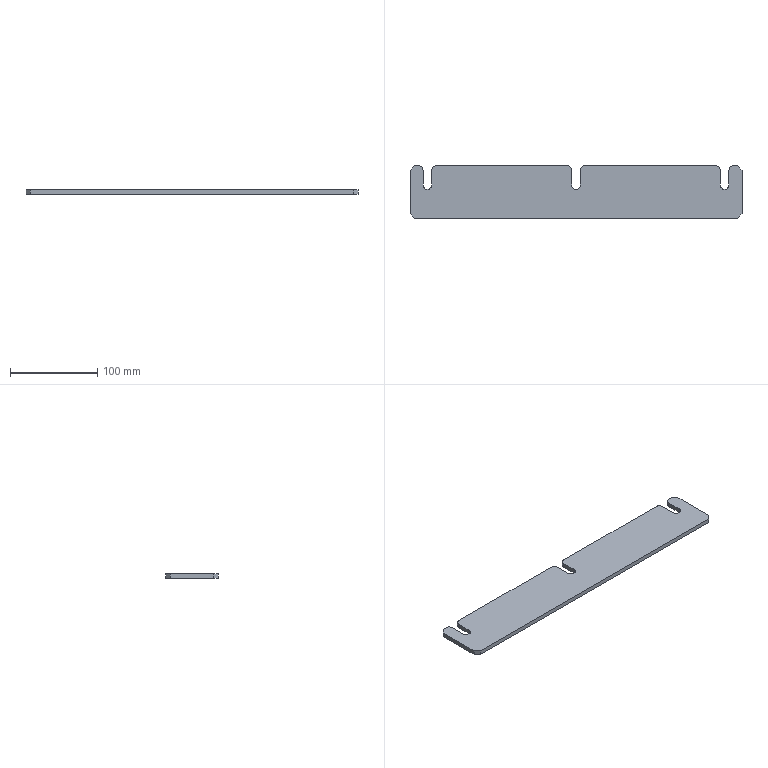Part | SolidWorks | features BaseBody 1 | 1 solid | 28 faces | box 380 x 60 x 5 mm | volume 109700 mm3 | plane 19 | cylinder 9 | commonest cylinder face diameters 10 x9
STEP:
#1=CARTESIAN_POINT('',(-185.,-30.,-5.));
#2=VERTEX_POINT('',#1);
#3=CARTESIAN_POINT('',(-190.,-25.,-5.));
#4=VERTEX_POINT('',#3);
#5=CARTESIAN_POINT('',(-190.,-25.,-5.));
#6=DIRECTION('',(-0.7071,0.7071,0.));
#7=VECTOR('',#6,1000.);
#8=LINE('',#5,#7);
#9=EDGE_CURVE('',#2,#4,#8,.T.);
#10=ORIENTED_EDGE('',*,*,#9,.F.);
#11=CARTESIAN_POINT('',(-185.,-30.,0.));
#12=VERTEX_POINT('',#11);
#13=CARTESIAN_POINT('',(-185.,-30.,-5.));
#14=DIRECTION('',(0.,0.,-1.));
#15=VECTOR('',#14,1000.);
#16=LINE('',#13,#15);
#17=EDGE_CURVE('',#12,#2,#16,.T.);
#18=ORIENTED_EDGE('',*,*,#17,.F.);
#19=CARTESIAN_POINT('',(-190.,-25.,0.));
#20=VERTEX_POINT('',#19);
#21=CARTESIAN_POINT('',(-107.5,-107.5,0.));
#22=DIRECTION('',(0.7071,-0.7071,0.));
#23=VECTOR('',#22,1000.);
#24=LINE('',#21,#23);
#25=EDGE_CURVE('',#20,#12,#24,.T.);
#26=ORIENTED_EDGE('',*,*,#25,.F.);
#27=CARTESIAN_POINT('',(-190.,-25.,-5.));
#28=DIRECTION('',(0.,0.,1.));
#29=VECTOR('',#28,1000.);
#30=LINE('',#27,#29);
#31=EDGE_CURVE('',#4,#20,#30,.T.);
#32=ORIENTED_EDGE('',*,*,#31,.F.);
#33=EDGE_LOOP('',(#10,#18,#26,#32));
#34=FACE_OUTER_BOUND('',#33,.T.);
#35=CARTESIAN_POINT('',(-190.,-25.,-5.));
#36=DIRECTION('',(0.7071,0.7071,0.));
#37=DIRECTION('',(0.,0.,-1.));
#38=AXIS2_PLACEMENT_3D('',#35,#36,#37);
#39=PLANE('',#38);
#40=ADVANCED_FACE('',(#34),#39,.F.);
#41=CARTESIAN_POINT('',(-190.,25.,-5.));
#42=VERTEX_POINT('',#41);
#43=CARTESIAN_POINT('',(-185.,30.,-5.));
#44=VERTEX_POINT('',#43);
#45=CARTESIAN_POINT('',(-185.,30.,-5.));
#46=DIRECTION('',(0.7071,0.7071,0.));
#47=VECTOR('',#46,1000.);
#48=LINE('',#45,#47);
#49=EDGE_CURVE('',#42,#44,#48,.T.);
#50=ORIENTED_EDGE('',*,*,#49,.F.);
#51=CARTESIAN_POINT('',(-190.,25.,0.));
#52=VERTEX_POINT('',#51);
#53=CARTESIAN_POINT('',(-190.,25.,-5.));
#54=DIRECTION('',(0.,0.,-1.));
#55=VECTOR('',#54,1000.);
#56=LINE('',#53,#55);
#57=EDGE_CURVE('',#52,#42,#56,.T.);
#58=ORIENTED_EDGE('',*,*,#57,.F.);
#59=CARTESIAN_POINT('',(-185.,30.,0.));
#60=VERTEX_POINT('',#59);
#61=CARTESIAN_POINT('',(-107.5,107.5,0.));
#62=DIRECTION('',(-0.7071,-0.7071,0.));
#63=VECTOR('',#62,1000.);
#64=LINE('',#61,#63);
#65=EDGE_CURVE('',#60,#52,#64,.T.);
#66=ORIENTED_EDGE('',*,*,#65,.F.);
#67=CARTESIAN_POINT('',(-185.,30.,-5.));
#68=DIRECTION('',(0.,0.,1.));
#69=VECTOR('',#68,1000.);
#70=LINE('',#67,#69);
#71=EDGE_CURVE('',#44,#60,#70,.T.);
#72=ORIENTED_EDGE('',*,*,#71,.F.);
#73=EDGE_LOOP('',(#50,#58,#66,#72));
#74=FACE_OUTER_BOUND('',#73,.T.);
#75=CARTESIAN_POINT('',(-185.,30.,-5.));
#76=DIRECTION('',(0.7071,-0.7071,0.));
#77=DIRECTION('',(0.,0.,-1.));
#78=AXIS2_PLACEMENT_3D('',#75,#76,#77);
#79=PLANE('',#78);
#80=ADVANCED_FACE('',(#74),#79,.F.);
#81=CARTESIAN_POINT('',(190.,-25.,-5.));
#82=VERTEX_POINT('',#81);
#83=CARTESIAN_POINT('',(185.,-30.,-5.));
#84=VERTEX_POINT('',#83);
#85=CARTESIAN_POINT('',(185.,-30.,-5.));
#86=DIRECTION('',(-0.7071,-0.7071,0.));
#87=VECTOR('',#86,1000.);
#88=LINE('',#85,#87);
#89=EDGE_CURVE('',#82,#84,#88,.T.);
#90=ORIENTED_EDGE('',*,*,#89,.F.);
#91=CARTESIAN_POINT('',(190.,-25.,0.));
#92=VERTEX_POINT('',#91);
#93=CARTESIAN_POINT('',(190.,-25.,-5.));
#94=DIRECTION('',(0.,0.,-1.));
#95=VECTOR('',#94,1000.);
#96=LINE('',#93,#95);
#97=EDGE_CURVE('',#92,#82,#96,.T.);
#98=ORIENTED_EDGE('',*,*,#97,.F.);
#99=CARTESIAN_POINT('',(185.,-30.,0.));
#100=VERTEX_POINT('',#99);
#101=CARTESIAN_POINT('',(107.5,-107.5,0.));
#102=DIRECTION('',(0.7071,0.7071,0.));
#103=VECTOR('',#102,1000.);
#104=LINE('',#101,#103);
#105=EDGE_CURVE('',#100,#92,#104,.T.);
#106=ORIENTED_EDGE('',*,*,#105,.F.);
#107=CARTESIAN_POINT('',(185.,-30.,-5.));
#108=DIRECTION('',(0.,0.,1.));
#109=VECTOR('',#108,1000.);
#110=LINE('',#107,#109);
#111=EDGE_CURVE('',#84,#100,#110,.T.);
#112=ORIENTED_EDGE('',*,*,#111,.F.);
#113=EDGE_LOOP('',(#90,#98,#106,#112));
#114=FACE_OUTER_BOUND('',#113,.T.);
#115=CARTESIAN_POINT('',(185.,-30.,-5.));
#116=DIRECTION('',(-0.7071,0.7071,0.));
#117=DIRECTION('',(0.,0.,1.));
#118=AXIS2_PLACEMENT_3D('',#115,#116,#117);
#119=PLANE('',#118);
#120=ADVANCED_FACE('',(#114),#119,.F.);
#121=CARTESIAN_POINT('',(185.,30.,-5.));
#122=VERTEX_POINT('',#121);
#123=CARTESIAN_POINT('',(190.,25.,-5.));
#124=VERTEX_POINT('',#123);
#125=CARTESIAN_POINT('',(190.,25.,-5.));
#126=DIRECTION('',(0.7071,-0.7071,0.));
#127=VECTOR('',#126,1000.);
#128=LINE('',#125,#127);
#129=EDGE_CURVE('',#122,#124,#128,.T.);
#130=ORIENTED_EDGE('',*,*,#129,.F.);
#131=CARTESIAN_POINT('',(185.,30.,0.));
#132=VERTEX_POINT('',#131);
#133=CARTESIAN_POINT('',(185.,30.,-5.));
#134=DIRECTION('',(0.,0.,-1.));
#135=VECTOR('',#134,1000.);
#136=LINE('',#133,#135);
#137=EDGE_CURVE('',#132,#122,#136,.T.);
#138=ORIENTED_EDGE('',*,*,#137,.F.);
#139=CARTESIAN_POINT('',(190.,25.,0.));
#140=VERTEX_POINT('',#139);
#141=CARTESIAN_POINT('',(107.5,107.5,0.));
#142=DIRECTION('',(-0.7071,0.7071,0.));
#143=VECTOR('',#142,1000.);
#144=LINE('',#141,#143);
#145=EDGE_CURVE('',#140,#132,#144,.T.);
#146=ORIENTED_EDGE('',*,*,#145,.F.);
#147=CARTESIAN_POINT('',(190.,25.,-5.));
#148=DIRECTION('',(0.,0.,1.));
#149=VECTOR('',#148,1000.);
#150=LINE('',#147,#149);
#151=EDGE_CURVE('',#124,#140,#150,.T.);
#152=ORIENTED_EDGE('',*,*,#151,.F.);
#153=EDGE_LOOP('',(#130,#138,#146,#152));
#154=FACE_OUTER_BOUND('',#153,.T.);
#155=CARTESIAN_POINT('',(190.,25.,-5.));
#156=DIRECTION('',(-0.7071,-0.7071,0.));
#157=DIRECTION('',(-0.7071,0.7071,0.));
#158=AXIS2_PLACEMENT_3D('',#155,#156,#157);
#159=PLANE('',#158);
#160=ADVANCED_FACE('',(#154),#159,.F.);
#161=CARTESIAN_POINT('',(-165.,25.,-5.));
#162=VERTEX_POINT('',#161);
#163=CARTESIAN_POINT('',(-160.,30.,-5.));
#164=VERTEX_POINT('',#163);
#165=CARTESIAN_POINT('',(-160.,25.,-5.));
#166=DIRECTION('',(0.,0.,-1.));
#167=DIRECTION('',(1.,0.,0.));
#168=AXIS2_PLACEMENT_3D('',#165,#166,#167);
#169=CIRCLE('',#168,5.);
#170=EDGE_CURVE('',#162,#164,#169,.T.);
#171=ORIENTED_EDGE('',*,*,#170,.F.);
#172=CARTESIAN_POINT('',(-165.,25.,0.));
#173=VERTEX_POINT('',#172);
#174=CARTESIAN_POINT('',(-165.,25.,-5.));
#175=DIRECTION('',(0.,0.,-1.));
#176=VECTOR('',#175,1000.);
#177=LINE('',#174,#176);
#178=EDGE_CURVE('',#173,#162,#177,.T.);
#179=ORIENTED_EDGE('',*,*,#178,.F.);
#180=CARTESIAN_POINT('',(-160.,30.,0.));
#181=VERTEX_POINT('',#180);
#182=CARTESIAN_POINT('',(-160.,25.,0.));
#183=DIRECTION('',(0.,0.,1.));
#184=DIRECTION('',(1.,0.,0.));
#185=AXIS2_PLACEMENT_3D('',#182,#183,#184);
#186=CIRCLE('',#185,5.);
#187=EDGE_CURVE('',#181,#173,#186,.T.);
#188=ORIENTED_EDGE('',*,*,#187,.F.);
#189=CARTESIAN_POINT('',(-160.,30.,0.));
#190=DIRECTION('',(0.,0.,1.));
#191=VECTOR('',#190,1000.);
#192=LINE('',#189,#191);
#193=EDGE_CURVE('',#164,#181,#192,.T.);
#194=ORIENTED_EDGE('',*,*,#193,.F.);
#195=EDGE_LOOP('',(#171,#179,#188,#194));
#196=FACE_OUTER_BOUND('',#195,.T.);
#197=CARTESIAN_POINT('',(-160.,25.,-5.));
#198=DIRECTION('',(0.,0.,-1.));
#199=DIRECTION('',(-1.,0.,0.));
#200=AXIS2_PLACEMENT_3D('',#197,#198,#199);
#201=CYLINDRICAL_SURFACE('',#200,5.);
#202=ADVANCED_FACE('',(#196),#201,.T.);
#203=CARTESIAN_POINT('',(-175.,25.,0.));
#204=VERTEX_POINT('',#203);
#205=CARTESIAN_POINT('',(-180.,30.,0.));
#206=VERTEX_POINT('',#205);
#207=CARTESIAN_POINT('',(-180.,25.,0.));
#208=DIRECTION('',(0.,0.,1.));
#209=DIRECTION('',(1.,0.,0.));
#210=AXIS2_PLACEMENT_3D('',#207,#208,#209);
#211=CIRCLE('',#210,5.);
#212=EDGE_CURVE('',#204,#206,#211,.T.);
#213=ORIENTED_EDGE('',*,*,#212,.F.);
#214=CARTESIAN_POINT('',(-175.,25.,-5.));
#215=VERTEX_POINT('',#214);
#216=CARTESIAN_POINT('',(-175.,25.,0.));
#217=DIRECTION('',(0.,0.,1.));
#218=VECTOR('',#217,1000.);
#219=LINE('',#216,#218);
#220=EDGE_CURVE('',#215,#204,#219,.T.);
#221=ORIENTED_EDGE('',*,*,#220,.F.);
#222=CARTESIAN_POINT('',(-180.,30.,-5.));
#223=VERTEX_POINT('',#222);
#224=CARTESIAN_POINT('',(-180.,25.,-5.));
#225=DIRECTION('',(0.,0.,-1.));
#226=DIRECTION('',(1.,0.,0.));
#227=AXIS2_PLACEMENT_3D('',#224,#225,#226);
#228=CIRCLE('',#227,5.);
#229=EDGE_CURVE('',#223,#215,#228,.T.);
#230=ORIENTED_EDGE('',*,*,#229,.F.);
#231=CARTESIAN_POINT('',(-180.,30.,-5.));
#232=DIRECTION('',(0.,0.,-1.));
#233=VECTOR('',#232,1000.);
#234=LINE('',#231,#233);
#235=EDGE_CURVE('',#206,#223,#234,.T.);
#236=ORIENTED_EDGE('',*,*,#235,.F.);
#237=EDGE_LOOP('',(#213,#221,#230,#236));
#238=FACE_OUTER_BOUND('',#237,.T.);
#239=CARTESIAN_POINT('',(-180.,25.,-5.));
#240=DIRECTION('',(0.,0.,1.));
#241=DIRECTION('',(1.,0.,0.));
#242=AXIS2_PLACEMENT_3D('',#239,#240,#241);
#243=CYLINDRICAL_SURFACE('',#242,5.);
#244=ADVANCED_FACE('',(#238),#243,.T.);
#245=CARTESIAN_POINT('',(5.,25.,-5.));
#246=VERTEX_POINT('',#245);
#247=CARTESIAN_POINT('',(10.,30.,-5.));
#248=VERTEX_POINT('',#247);
#249=CARTESIAN_POINT('',(10.,25.,-5.));
#250=DIRECTION('',(0.,0.,-1.));
#251=DIRECTION('',(1.,0.,0.));
#252=AXIS2_PLACEMENT_3D('',#249,#250,#251);
#253=CIRCLE('',#252,5.);
#254=EDGE_CURVE('',#246,#248,#253,.T.);
#255=ORIENTED_EDGE('',*,*,#254,.F.);
#256=CARTESIAN_POINT('',(5.,25.,0.));
#257=VERTEX_POINT('',#256);
#258=CARTESIAN_POINT('',(5.,25.,-5.));
#259=DIRECTION('',(0.,0.,-1.));
#260=VECTOR('',#259,1000.);
#261=LINE('',#258,#260);
#262=EDGE_CURVE('',#257,#246,#261,.T.);
#263=ORIENTED_EDGE('',*,*,#262,.F.);
#264=CARTESIAN_POINT('',(10.,30.,0.));
#265=VERTEX_POINT('',#264);
#266=CARTESIAN_POINT('',(10.,25.,0.));
#267=DIRECTION('',(0.,0.,1.));
#268=DIRECTION('',(1.,0.,0.));
#269=AXIS2_PLACEMENT_3D('',#266,#267,#268);
#270=CIRCLE('',#269,5.);
#271=EDGE_CURVE('',#265,#257,#270,.T.);
#272=ORIENTED_EDGE('',*,*,#271,.F.);
#273=CARTESIAN_POINT('',(10.,30.,0.));
#274=DIRECTION('',(0.,0.,1.));
#275=VECTOR('',#274,1000.);
#276=LINE('',#273,#275);
#277=EDGE_CURVE('',#248,#265,#276,.T.);
#278=ORIENTED_EDGE('',*,*,#277,.F.);
#279=EDGE_LOOP('',(#255,#263,#272,#278));
#280=FACE_OUTER_BOUND('',#279,.T.);
#281=CARTESIAN_POINT('',(10.,25.,-5.));
#282=DIRECTION('',(0.,0.,-1.));
#283=DIRECTION('',(-1.,0.,0.));
#284=AXIS2_PLACEMENT_3D('',#281,#282,#283);
#285=CYLINDRICAL_SURFACE('',#284,5.);
#286=ADVANCED_FACE('',(#280),#285,.T.);
#287=CARTESIAN_POINT('',(-5.,25.,0.));
#288=VERTEX_POINT('',#287);
#289=CARTESIAN_POINT('',(-10.,30.,0.));
#290=VERTEX_POINT('',#289);
#291=CARTESIAN_POINT('',(-10.,25.,0.));
#292=DIRECTION('',(0.,0.,1.));
#293=DIRECTION('',(1.,0.,0.));
#294=AXIS2_PLACEMENT_3D('',#291,#292,#293);
#295=CIRCLE('',#294,5.);
#296=EDGE_CURVE('',#288,#290,#295,.T.);
#297=ORIENTED_EDGE('',*,*,#296,.F.);
#298=CARTESIAN_POINT('',(-5.,25.,-5.));
#299=VERTEX_POINT('',#298);
#300=CARTESIAN_POINT('',(-5.,25.,0.));
#301=DIRECTION('',(0.,0.,1.));
#302=VECTOR('',#301,1000.);
#303=LINE('',#300,#302);
#304=EDGE_CURVE('',#299,#288,#303,.T.);
#305=ORIENTED_EDGE('',*,*,#304,.F.);
#306=CARTESIAN_POINT('',(-10.,30.,-5.));
#307=VERTEX_POINT('',#306);
#308=CARTESIAN_POINT('',(-10.,25.,-5.));
#309=DIRECTION('',(0.,0.,-1.));
#310=DIRECTION('',(1.,0.,0.));
#311=AXIS2_PLACEMENT_3D('',#308,#309,#310);
#312=CIRCLE('',#311,5.);
#313=EDGE_CURVE('',#307,#299,#312,.T.);
#314=ORIENTED_EDGE('',*,*,#313,.F.);
#315=CARTESIAN_POINT('',(-10.,30.,-5.));
#316=DIRECTION('',(0.,0.,-1.));
#317=VECTOR('',#316,1000.);
#318=LINE('',#315,#317);
#319=EDGE_CURVE('',#290,#307,#318,.T.);
#320=ORIENTED_EDGE('',*,*,#319,.F.);
#321=EDGE_LOOP('',(#297,#305,#314,#320));
#322=FACE_OUTER_BOUND('',#321,.T.);
#323=CARTESIAN_POINT('',(-10.,25.,-5.));
#324=DIRECTION('',(0.,0.,1.));
#325=DIRECTION('',(1.,0.,0.));
#326=AXIS2_PLACEMENT_3D('',#323,#324,#325);
#327=CYLINDRICAL_SURFACE('',#326,5.);
#328=ADVANCED_FACE('',(#322),#327,.T.);
#329=CARTESIAN_POINT('',(175.,25.,-5.));
#330=VERTEX_POINT('',#329);
#331=CARTESIAN_POINT('',(180.,30.,-5.));
#332=VERTEX_POINT('',#331);
#333=CARTESIAN_POINT('',(180.,25.,-5.));
#334=DIRECTION('',(0.,0.,-1.));
#335=DIRECTION('',(1.,0.,0.));
#336=AXIS2_PLACEMENT_3D('',#333,#334,#335);
#337=CIRCLE('',#336,5.);
#338=EDGE_CURVE('',#330,#332,#337,.T.);
#339=ORIENTED_EDGE('',*,*,#338,.F.);
#340=CARTESIAN_POINT('',(175.,25.,0.));
#341=VERTEX_POINT('',#340);
#342=CARTESIAN_POINT('',(175.,25.,-5.));
#343=DIRECTION('',(0.,0.,-1.));
#344=VECTOR('',#343,1000.);
#345=LINE('',#342,#344);
#346=EDGE_CURVE('',#341,#330,#345,.T.);
#347=ORIENTED_EDGE('',*,*,#346,.F.);
#348=CARTESIAN_POINT('',(180.,30.,0.));
#349=VERTEX_POINT('',#348);
#350=CARTESIAN_POINT('',(180.,25.,0.));
#351=DIRECTION('',(0.,0.,1.));
#352=DIRECTION('',(1.,0.,0.));
#353=AXIS2_PLACEMENT_3D('',#350,#351,#352);
#354=CIRCLE('',#353,5.);
#355=EDGE_CURVE('',#349,#341,#354,.T.);
#356=ORIENTED_EDGE('',*,*,#355,.F.);
#357=CARTESIAN_POINT('',(180.,30.,0.));
#358=DIRECTION('',(0.,0.,1.));
#359=VECTOR('',#358,1000.);
#360=LINE('',#357,#359);
#361=EDGE_CURVE('',#332,#349,#360,.T.);
#362=ORIENTED_EDGE('',*,*,#361,.F.);
#363=EDGE_LOOP('',(#339,#347,#356,#362));
#364=FACE_OUTER_BOUND('',#363,.T.);
#365=CARTESIAN_POINT('',(180.,25.,-5.));
#366=DIRECTION('',(0.,0.,-1.));
#367=DIRECTION('',(-1.,0.,0.));
#368=AXIS2_PLACEMENT_3D('',#365,#366,#367);
#369=CYLINDRICAL_SURFACE('',#368,5.);
#370=ADVANCED_FACE('',(#364),#369,.T.);
#371=CARTESIAN_POINT('',(165.,25.,0.));
#372=VERTEX_POINT('',#371);
#373=CARTESIAN_POINT('',(160.,30.,0.));
#374=VERTEX_POINT('',#373);
#375=CARTESIAN_POINT('',(160.,25.,0.));
#376=DIRECTION('',(0.,0.,1.));
#377=DIRECTION('',(1.,0.,0.));
#378=AXIS2_PLACEMENT_3D('',#375,#376,#377);
#379=CIRCLE('',#378,5.);
#380=EDGE_CURVE('',#372,#374,#379,.T.);
#381=ORIENTED_EDGE('',*,*,#380,.F.);
#382=CARTESIAN_POINT('',(165.,25.,-5.));
#383=VERTEX_POINT('',#382);
#384=CARTESIAN_POINT('',(165.,25.,0.));
#385=DIRECTION('',(0.,0.,1.));
#386=VECTOR('',#385,1000.);
#387=LINE('',#384,#386);
#388=EDGE_CURVE('',#383,#372,#387,.T.);
#389=ORIENTED_EDGE('',*,*,#388,.F.);
#390=CARTESIAN_POINT('',(160.,30.,-5.));
#391=VERTEX_POINT('',#390);
#392=CARTESIAN_POINT('',(160.,25.,-5.));
#393=DIRECTION('',(0.,0.,-1.));
#394=DIRECTION('',(1.,0.,0.));
#395=AXIS2_PLACEMENT_3D('',#392,#393,#394);
#396=CIRCLE('',#395,5.);
#397=EDGE_CURVE('',#391,#383,#396,.T.);
#398=ORIENTED_EDGE('',*,*,#397,.F.);
#399=CARTESIAN_POINT('',(160.,30.,-5.));
#400=DIRECTION('',(0.,0.,-1.));
#401=VECTOR('',#400,1000.);
#402=LINE('',#399,#401);
#403=EDGE_CURVE('',#374,#391,#402,.T.);
#404=ORIENTED_EDGE('',*,*,#403,.F.);
#405=EDGE_LOOP('',(#381,#389,#398,#404));
#406=FACE_OUTER_BOUND('',#405,.T.);
#407=CARTESIAN_POINT('',(160.,25.,-5.));
#408=DIRECTION('',(0.,0.,1.));
#409=DIRECTION('',(1.,0.,0.));
#410=AXIS2_PLACEMENT_3D('',#407,#408,#409);
#411=CYLINDRICAL_SURFACE('',#410,5.);
#412=ADVANCED_FACE('',(#406),#411,.T.);
#413=CARTESIAN_POINT('',(-175.,8.,-5.));
#414=VERTEX_POINT('',#413);
#415=CARTESIAN_POINT('',(-175.,30.,-5.));
#416=DIRECTION('',(0.,1.,0.));
#417=VECTOR('',#416,1000.);
#418=LINE('',#415,#417);
#419=EDGE_CURVE('',#414,#215,#418,.T.);
#420=ORIENTED_EDGE('',*,*,#419,.T.);
#421=ORIENTED_EDGE('',*,*,#220,.T.);
#422=CARTESIAN_POINT('',(-175.,8.,0.));
#423=VERTEX_POINT('',#422);
#424=CARTESIAN_POINT('',(-175.,30.,0.));
#425=DIRECTION('',(0.,-1.,0.));
#426=VECTOR('',#425,1000.);
#427=LINE('',#424,#426);
#428=EDGE_CURVE('',#204,#423,#427,.T.);
#429=ORIENTED_EDGE('',*,*,#428,.T.);
#430=CARTESIAN_POINT('',(-175.,8.,-5.001));
#431=DIRECTION('',(0.,0.,1.));
#432=VECTOR('',#431,1000.);
#433=LINE('',#430,#432);
#434=EDGE_CURVE('',#414,#423,#433,.T.);
#435=ORIENTED_EDGE('',*,*,#434,.F.);
#436=EDGE_LOOP('',(#420,#421,#429,#435));
#437=FACE_OUTER_BOUND('',#436,.T.);
#438=CARTESIAN_POINT('',(-175.,30.,-5.001));
#439=DIRECTION('',(-1.,0.,0.));
#440=DIRECTION('',(0.,0.,1.));
#441=AXIS2_PLACEMENT_3D('',#438,#439,#440);
#442=PLANE('',#441);
#443=ADVANCED_FACE('',(#437),#442,.F.);
#444=CARTESIAN_POINT('',(-165.,8.,0.));
#445=VERTEX_POINT('',#444);
#446=CARTESIAN_POINT('',(-170.,8.,0.));
#447=DIRECTION('',(0.,0.,1.));
#448=DIRECTION('',(1.,0.,0.));
#449=AXIS2_PLACEMENT_3D('',#446,#447,#448);
#450=CIRCLE('',#449,5.);
#451=EDGE_CURVE('',#423,#445,#450,.T.);
#452=ORIENTED_EDGE('',*,*,#451,.T.);
#453=CARTESIAN_POINT('',(-165.,8.,-5.));
#454=VERTEX_POINT('',#453);
#455=CARTESIAN_POINT('',(-165.,8.,-5.001));
#456=DIRECTION('',(0.,0.,1.));
#457=VECTOR('',#456,1000.);
#458=LINE('',#455,#457);
#459=EDGE_CURVE('',#454,#445,#458,.T.);
#460=ORIENTED_EDGE('',*,*,#459,.F.);
#461=CARTESIAN_POINT('',(-170.,8.,-5.));
#462=DIRECTION('',(0.,0.,-1.));
#463=DIRECTION('',(1.,0.,0.));
#464=AXIS2_PLACEMENT_3D('',#461,#462,#463);
#465=CIRCLE('',#464,5.);
#466=EDGE_CURVE('',#454,#414,#465,.T.);
#467=ORIENTED_EDGE('',*,*,#466,.T.);
#468=ORIENTED_EDGE('',*,*,#434,.T.);
#469=EDGE_LOOP('',(#452,#460,#467,#468));
#470=FACE_OUTER_BOUND('',#469,.T.);
#471=CARTESIAN_POINT('',(-170.,8.,-5.001));
#472=DIRECTION('',(0.,0.,1.));
#473=DIRECTION('',(1.,0.,0.));
#474=AXIS2_PLACEMENT_3D('',#471,#472,#473);
#475=CYLINDRICAL_SURFACE('',#474,5.);
#476=ADVANCED_FACE('',(#470),#475,.F.);
#477=CARTESIAN_POINT('',(-165.,30.,0.));
#478=DIRECTION('',(0.,1.,0.));
#479=VECTOR('',#478,1000.);
#480=LINE('',#477,#479);
#481=EDGE_CURVE('',#445,#173,#480,.T.);
#482=ORIENTED_EDGE('',*,*,#481,.T.);
#483=ORIENTED_EDGE('',*,*,#178,.T.);
#484=CARTESIAN_POINT('',(-165.,30.,-5.));
#485=DIRECTION('',(0.,-1.,0.));
#486=VECTOR('',#485,1000.);
#487=LINE('',#484,#486);
#488=EDGE_CURVE('',#162,#454,#487,.T.);
#489=ORIENTED_EDGE('',*,*,#488,.T.);
#490=ORIENTED_EDGE('',*,*,#459,.T.);
#491=EDGE_LOOP('',(#482,#483,#489,#490));
#492=FACE_OUTER_BOUND('',#491,.T.);
#493=CARTESIAN_POINT('',(-165.,30.,-5.001));
#494=DIRECTION('',(1.,0.,0.));
#495=DIRECTION('',(0.,1.,0.));
#496=AXIS2_PLACEMENT_3D('',#493,#494,#495);
#497=PLANE('',#496);
#498=ADVANCED_FACE('',(#492),#497,.F.);
#499=CARTESIAN_POINT('',(-5.,8.,-5.));
#500=VERTEX_POINT('',#499);
#501=CARTESIAN_POINT('',(-5.,30.,-5.));
#502=DIRECTION('',(0.,1.,0.));
#503=VECTOR('',#502,1000.);
#504=LINE('',#501,#503);
#505=EDGE_CURVE('',#500,#299,#504,.T.);
#506=ORIENTED_EDGE('',*,*,#505,.T.);
#507=ORIENTED_EDGE('',*,*,#304,.T.);
#508=CARTESIAN_POINT('',(-5.,8.,0.));
#509=VERTEX_POINT('',#508);
#510=CARTESIAN_POINT('',(-5.,30.,0.));
#511=DIRECTION('',(0.,-1.,0.));
#512=VECTOR('',#511,1000.);
#513=LINE('',#510,#512);
#514=EDGE_CURVE('',#288,#509,#513,.T.);
#515=ORIENTED_EDGE('',*,*,#514,.T.);
#516=CARTESIAN_POINT('',(-5.,8.,-5.001));
#517=DIRECTION('',(0.,0.,1.));
#518=VECTOR('',#517,1000.);
#519=LINE('',#516,#518);
#520=EDGE_CURVE('',#500,#509,#519,.T.);
#521=ORIENTED_EDGE('',*,*,#520,.F.);
#522=EDGE_LOOP('',(#506,#507,#515,#521));
#523=FACE_OUTER_BOUND('',#522,.T.);
#524=CARTESIAN_POINT('',(-5.,30.,-5.001));
#525=DIRECTION('',(-1.,0.,0.));
#526=DIRECTION('',(0.,0.,1.));
#527=AXIS2_PLACEMENT_3D('',#524,#525,#526);
#528=PLANE('',#527);
#529=ADVANCED_FACE('',(#523),#528,.F.);
#530=CARTESIAN_POINT('',(5.,8.,0.));
#531=VERTEX_POINT('',#530);
#532=CARTESIAN_POINT('',(0.,8.,0.));
#533=DIRECTION('',(0.,0.,1.));
#534=DIRECTION('',(1.,0.,0.));
#535=AXIS2_PLACEMENT_3D('',#532,#533,#534);
#536=CIRCLE('',#535,5.);
#537=EDGE_CURVE('',#509,#531,#536,.T.);
#538=ORIENTED_EDGE('',*,*,#537,.T.);
#539=CARTESIAN_POINT('',(5.,8.,-5.));
#540=VERTEX_POINT('',#539);
#541=CARTESIAN_POINT('',(5.,8.,-5.001));
#542=DIRECTION('',(0.,0.,1.));
#543=VECTOR('',#542,1000.);
#544=LINE('',#541,#543);
#545=EDGE_CURVE('',#540,#531,#544,.T.);
#546=ORIENTED_EDGE('',*,*,#545,.F.);
#547=CARTESIAN_POINT('',(0.,8.,-5.));
#548=DIRECTION('',(0.,0.,-1.));
#549=DIRECTION('',(1.,0.,0.));
#550=AXIS2_PLACEMENT_3D('',#547,#548,#549);
#551=CIRCLE('',#550,5.);
#552=EDGE_CURVE('',#540,#500,#551,.T.);
#553=ORIENTED_EDGE('',*,*,#552,.T.);
#554=ORIENTED_EDGE('',*,*,#520,.T.);
#555=EDGE_LOOP('',(#538,#546,#553,#554));
#556=FACE_OUTER_BOUND('',#555,.T.);
#557=CARTESIAN_POINT('',(0.,8.,-5.001));
#558=DIRECTION('',(0.,0.,1.));
#559=DIRECTION('',(1.,0.,0.));
#560=AXIS2_PLACEMENT_3D('',#557,#558,#559);
#561=CYLINDRICAL_SURFACE('',#560,5.);
#562=ADVANCED_FACE('',(#556),#561,.F.);
#563=CARTESIAN_POINT('',(5.,30.,0.));
#564=DIRECTION('',(0.,1.,0.));
#565=VECTOR('',#564,1000.);
#566=LINE('',#563,#565);
#567=EDGE_CURVE('',#531,#257,#566,.T.);
#568=ORIENTED_EDGE('',*,*,#567,.T.);
#569=ORIENTED_EDGE('',*,*,#262,.T.);
#570=CARTESIAN_POINT('',(5.,30.,-5.));
#571=DIRECTION('',(0.,-1.,0.));
#572=VECTOR('',#571,1000.);
#573=LINE('',#570,#572);
#574=EDGE_CURVE('',#246,#540,#573,.T.);
#575=ORIENTED_EDGE('',*,*,#574,.T.);
#576=ORIENTED_EDGE('',*,*,#545,.T.);
#577=EDGE_LOOP('',(#568,#569,#575,#576));
#578=FACE_OUTER_BOUND('',#577,.T.);
#579=CARTESIAN_POINT('',(5.,30.,-5.001));
#580=DIRECTION('',(1.,0.,0.));
#581=DIRECTION('',(0.,-1.,0.));
#582=AXIS2_PLACEMENT_3D('',#579,#580,#581);
#583=PLANE('',#582);
#584=ADVANCED_FACE('',(#578),#583,.F.);
#585=CARTESIAN_POINT('',(165.,8.,-5.));
#586=VERTEX_POINT('',#585);
#587=CARTESIAN_POINT('',(165.,30.,-5.));
#588=DIRECTION('',(0.,1.,0.));
#589=VECTOR('',#588,1000.);
#590=LINE('',#587,#589);
#591=EDGE_CURVE('',#586,#383,#590,.T.);
#592=ORIENTED_EDGE('',*,*,#591,.T.);
#593=ORIENTED_EDGE('',*,*,#388,.T.);
#594=CARTESIAN_POINT('',(165.,8.,0.));
#595=VERTEX_POINT('',#594);
#596=CARTESIAN_POINT('',(165.,30.,0.));
#597=DIRECTION('',(0.,-1.,0.));
#598=VECTOR('',#597,1000.);
#599=LINE('',#596,#598);
#600=EDGE_CURVE('',#372,#595,#599,.T.);
#601=ORIENTED_EDGE('',*,*,#600,.T.);
#602=CARTESIAN_POINT('',(165.,8.,-5.001));
#603=DIRECTION('',(0.,0.,1.));
#604=VECTOR('',#603,1000.);
#605=LINE('',#602,#604);
#606=EDGE_CURVE('',#586,#595,#605,.T.);
#607=ORIENTED_EDGE('',*,*,#606,.F.);
#608=EDGE_LOOP('',(#592,#593,#601,#607));
#609=FACE_OUTER_BOUND('',#608,.T.);
#610=CARTESIAN_POINT('',(165.,30.,-5.001));
#611=DIRECTION('',(-1.,0.,0.));
#612=DIRECTION('',(0.,0.,1.));
#613=AXIS2_PLACEMENT_3D('',#610,#611,#612);
#614=PLANE('',#613);
#615=ADVANCED_FACE('',(#609),#614,.F.);
#616=CARTESIAN_POINT('',(175.,8.,0.));
#617=VERTEX_POINT('',#616);
#618=CARTESIAN_POINT('',(170.,8.,0.));
#619=DIRECTION('',(0.,0.,1.));
#620=DIRECTION('',(1.,0.,0.));
#621=AXIS2_PLACEMENT_3D('',#618,#619,#620);
#622=CIRCLE('',#621,5.);
#623=EDGE_CURVE('',#595,#617,#622,.T.);
#624=ORIENTED_EDGE('',*,*,#623,.T.);
#625=CARTESIAN_POINT('',(175.,8.,-5.));
#626=VERTEX_POINT('',#625);
#627=CARTESIAN_POINT('',(175.,8.,-5.001));
#628=DIRECTION('',(0.,0.,1.));
#629=VECTOR('',#628,1000.);
#630=LINE('',#627,#629);
#631=EDGE_CURVE('',#626,#617,#630,.T.);
#632=ORIENTED_EDGE('',*,*,#631,.F.);
#633=CARTESIAN_POINT('',(170.,8.,-5.));
#634=DIRECTION('',(0.,0.,-1.));
#635=DIRECTION('',(1.,0.,0.));
#636=AXIS2_PLACEMENT_3D('',#633,#634,#635);
#637=CIRCLE('',#636,5.);
#638=EDGE_CURVE('',#626,#586,#637,.T.);
#639=ORIENTED_EDGE('',*,*,#638,.T.);
#640=ORIENTED_EDGE('',*,*,#606,.T.);
#641=EDGE_LOOP('',(#624,#632,#639,#640));
#642=FACE_OUTER_BOUND('',#641,.T.);
#643=CARTESIAN_POINT('',(170.,8.,-5.001));
#644=DIRECTION('',(0.,0.,1.));
#645=DIRECTION('',(1.,0.,0.));
#646=AXIS2_PLACEMENT_3D('',#643,#644,#645);
#647=CYLINDRICAL_SURFACE('',#646,5.);
#648=ADVANCED_FACE('',(#642),#647,.F.);
#649=CARTESIAN_POINT('',(175.,30.,0.));
#650=DIRECTION('',(0.,1.,0.));
#651=VECTOR('',#650,1000.);
#652=LINE('',#649,#651);
#653=EDGE_CURVE('',#617,#341,#652,.T.);
#654=ORIENTED_EDGE('',*,*,#653,.T.);
#655=ORIENTED_EDGE('',*,*,#346,.T.);
#656=CARTESIAN_POINT('',(175.,30.,-5.));
#657=DIRECTION('',(0.,-1.,0.));
#658=VECTOR('',#657,1000.);
#659=LINE('',#656,#658);
#660=EDGE_CURVE('',#330,#626,#659,.T.);
#661=ORIENTED_EDGE('',*,*,#660,.T.);
#662=ORIENTED_EDGE('',*,*,#631,.T.);
#663=EDGE_LOOP('',(#654,#655,#661,#662));
#664=FACE_OUTER_BOUND('',#663,.T.);
#665=CARTESIAN_POINT('',(175.,30.,-5.001));
#666=DIRECTION('',(1.,0.,0.));
#667=DIRECTION('',(0.,1.,0.));
#668=AXIS2_PLACEMENT_3D('',#665,#666,#667);
#669=PLANE('',#668);
#670=ADVANCED_FACE('',(#664),#669,.F.);
#671=CARTESIAN_POINT('',(190.,-30.,0.));
#672=DIRECTION('',(0.,1.,0.));
#673=VECTOR('',#672,1000.);
#674=LINE('',#671,#673);
#675=EDGE_CURVE('',#92,#140,#674,.T.);
#676=ORIENTED_EDGE('',*,*,#675,.T.);
#677=ORIENTED_EDGE('',*,*,#145,.T.);
#678=CARTESIAN_POINT('',(190.,30.,0.));
#679=DIRECTION('',(-1.,0.,0.));
#680=VECTOR('',#679,1000.);
#681=LINE('',#678,#680);
#682=EDGE_CURVE('',#132,#349,#681,.T.);
#683=ORIENTED_EDGE('',*,*,#682,.T.);
#684=ORIENTED_EDGE('',*,*,#355,.T.);
#685=ORIENTED_EDGE('',*,*,#653,.F.);
#686=ORIENTED_EDGE('',*,*,#623,.F.);
#687=ORIENTED_EDGE('',*,*,#600,.F.);
#688=ORIENTED_EDGE('',*,*,#380,.T.);
#689=CARTESIAN_POINT('',(190.,30.,0.));
#690=DIRECTION('',(-1.,0.,0.));
#691=VECTOR('',#690,1000.);
#692=LINE('',#689,#691);
#693=EDGE_CURVE('',#374,#265,#692,.T.);
#694=ORIENTED_EDGE('',*,*,#693,.T.);
#695=ORIENTED_EDGE('',*,*,#271,.T.);
#696=ORIENTED_EDGE('',*,*,#567,.F.);
#697=ORIENTED_EDGE('',*,*,#537,.F.);
#698=ORIENTED_EDGE('',*,*,#514,.F.);
#699=ORIENTED_EDGE('',*,*,#296,.T.);
#700=CARTESIAN_POINT('',(190.,30.,0.));
#701=DIRECTION('',(-1.,0.,0.));
#702=VECTOR('',#701,1000.);
#703=LINE('',#700,#702);
#704=EDGE_CURVE('',#290,#181,#703,.T.);
#705=ORIENTED_EDGE('',*,*,#704,.T.);
#706=ORIENTED_EDGE('',*,*,#187,.T.);
#707=ORIENTED_EDGE('',*,*,#481,.F.);
#708=ORIENTED_EDGE('',*,*,#451,.F.);
#709=ORIENTED_EDGE('',*,*,#428,.F.);
#710=ORIENTED_EDGE('',*,*,#212,.T.);
#711=CARTESIAN_POINT('',(190.,30.,0.));
#712=DIRECTION('',(-1.,0.,0.));
#713=VECTOR('',#712,1000.);
#714=LINE('',#711,#713);
#715=EDGE_CURVE('',#206,#60,#714,.T.);
#716=ORIENTED_EDGE('',*,*,#715,.T.);
#717=ORIENTED_EDGE('',*,*,#65,.T.);
#718=CARTESIAN_POINT('',(-190.,-30.,0.));
#719=DIRECTION('',(0.,-1.,0.));
#720=VECTOR('',#719,1000.);
#721=LINE('',#718,#720);
#722=EDGE_CURVE('',#52,#20,#721,.T.);
#723=ORIENTED_EDGE('',*,*,#722,.T.);
#724=ORIENTED_EDGE('',*,*,#25,.T.);
#725=CARTESIAN_POINT('',(190.,-30.,0.));
#726=DIRECTION('',(1.,0.,0.));
#727=VECTOR('',#726,1000.);
#728=LINE('',#725,#727);
#729=EDGE_CURVE('',#12,#100,#728,.T.);
#730=ORIENTED_EDGE('',*,*,#729,.T.);
#731=ORIENTED_EDGE('',*,*,#105,.T.);
#732=EDGE_LOOP('',(#676,#677,#683,#684,#685,#686,#687,#688,#694,#695,#696,#697,#698,#699,#705,#706,#707,#708,#709,#710,#716,#717,#723,#724,#730,#731));
#733=FACE_OUTER_BOUND('',#732,.T.);
#734=CARTESIAN_POINT('',(0.,0.,0.));
#735=DIRECTION('',(0.,0.,1.));
#736=DIRECTION('',(1.,0.,0.));
#737=AXIS2_PLACEMENT_3D('',#734,#735,#736);
#738=PLANE('',#737);
#739=ADVANCED_FACE('',(#733),#738,.T.);
#740=CARTESIAN_POINT('',(190.,30.,-5.));
#741=DIRECTION('',(-1.,0.,0.));
#742=VECTOR('',#741,1000.);
#743=LINE('',#740,#742);
#744=EDGE_CURVE('',#122,#332,#743,.T.);
#745=ORIENTED_EDGE('',*,*,#744,.F.);
#746=ORIENTED_EDGE('',*,*,#129,.T.);
#747=CARTESIAN_POINT('',(190.,-30.,-5.));
#748=DIRECTION('',(0.,1.,0.));
#749=VECTOR('',#748,1000.);
#750=LINE('',#747,#749);
#751=EDGE_CURVE('',#82,#124,#750,.T.);
#752=ORIENTED_EDGE('',*,*,#751,.F.);
#753=ORIENTED_EDGE('',*,*,#89,.T.);
#754=CARTESIAN_POINT('',(190.,-30.,-5.));
#755=DIRECTION('',(1.,0.,0.));
#756=VECTOR('',#755,1000.);
#757=LINE('',#754,#756);
#758=EDGE_CURVE('',#2,#84,#757,.T.);
#759=ORIENTED_EDGE('',*,*,#758,.F.);
#760=ORIENTED_EDGE('',*,*,#9,.T.);
#761=CARTESIAN_POINT('',(-190.,-30.,-5.));
#762=DIRECTION('',(0.,-1.,0.));
#763=VECTOR('',#762,1000.);
#764=LINE('',#761,#763);
#765=EDGE_CURVE('',#42,#4,#764,.T.);
#766=ORIENTED_EDGE('',*,*,#765,.F.);
#767=ORIENTED_EDGE('',*,*,#49,.T.);
#768=CARTESIAN_POINT('',(190.,30.,-5.));
#769=DIRECTION('',(-1.,0.,0.));
#770=VECTOR('',#769,1000.);
#771=LINE('',#768,#770);
#772=EDGE_CURVE('',#223,#44,#771,.T.);
#773=ORIENTED_EDGE('',*,*,#772,.F.);
#774=ORIENTED_EDGE('',*,*,#229,.T.);
#775=ORIENTED_EDGE('',*,*,#419,.F.);
#776=ORIENTED_EDGE('',*,*,#466,.F.);
#777=ORIENTED_EDGE('',*,*,#488,.F.);
#778=ORIENTED_EDGE('',*,*,#170,.T.);
#779=CARTESIAN_POINT('',(190.,30.,-5.));
#780=DIRECTION('',(-1.,0.,0.));
#781=VECTOR('',#780,1000.);
#782=LINE('',#779,#781);
#783=EDGE_CURVE('',#307,#164,#782,.T.);
#784=ORIENTED_EDGE('',*,*,#783,.F.);
#785=ORIENTED_EDGE('',*,*,#313,.T.);
#786=ORIENTED_EDGE('',*,*,#505,.F.);
#787=ORIENTED_EDGE('',*,*,#552,.F.);
#788=ORIENTED_EDGE('',*,*,#574,.F.);
#789=ORIENTED_EDGE('',*,*,#254,.T.);
#790=CARTESIAN_POINT('',(190.,30.,-5.));
#791=DIRECTION('',(-1.,0.,0.));
#792=VECTOR('',#791,1000.);
#793=LINE('',#790,#792);
#794=EDGE_CURVE('',#391,#248,#793,.T.);
#795=ORIENTED_EDGE('',*,*,#794,.F.);
#796=ORIENTED_EDGE('',*,*,#397,.T.);
#797=ORIENTED_EDGE('',*,*,#591,.F.);
#798=ORIENTED_EDGE('',*,*,#638,.F.);
#799=ORIENTED_EDGE('',*,*,#660,.F.);
#800=ORIENTED_EDGE('',*,*,#338,.T.);
#801=EDGE_LOOP('',(#745,#746,#752,#753,#759,#760,#766,#767,#773,#774,#775,#776,#777,#778,#784,#785,#786,#787,#788,#789,#795,#796,#797,#798,#799,#800));
#802=FACE_OUTER_BOUND('',#801,.T.);
#803=CARTESIAN_POINT('',(0.,0.,-5.));
#804=DIRECTION('',(0.,0.,1.));
#805=DIRECTION('',(1.,0.,0.));
#806=AXIS2_PLACEMENT_3D('',#803,#804,#805);
#807=PLANE('',#806);
#808=ADVANCED_FACE('',(#802),#807,.F.);
#809=ORIENTED_EDGE('',*,*,#758,.T.);
#810=ORIENTED_EDGE('',*,*,#111,.T.);
#811=ORIENTED_EDGE('',*,*,#729,.F.);
#812=ORIENTED_EDGE('',*,*,#17,.T.);
#813=EDGE_LOOP('',(#809,#810,#811,#812));
#814=FACE_OUTER_BOUND('',#813,.T.);
#815=CARTESIAN_POINT('',(190.,-30.,-5.));
#816=DIRECTION('',(0.,-1.,0.));
#817=DIRECTION('',(0.,0.,-1.));
#818=AXIS2_PLACEMENT_3D('',#815,#816,#817);
#819=PLANE('',#818);
#820=ADVANCED_FACE('',(#814),#819,.T.);
#821=ORIENTED_EDGE('',*,*,#751,.T.);
#822=ORIENTED_EDGE('',*,*,#151,.T.);
#823=ORIENTED_EDGE('',*,*,#675,.F.);
#824=ORIENTED_EDGE('',*,*,#97,.T.);
#825=EDGE_LOOP('',(#821,#822,#823,#824));
#826=FACE_OUTER_BOUND('',#825,.T.);
#827=CARTESIAN_POINT('',(190.,-30.,-5.));
#828=DIRECTION('',(1.,0.,0.));
#829=DIRECTION('',(0.,1.,0.));
#830=AXIS2_PLACEMENT_3D('',#827,#828,#829);
#831=PLANE('',#830);
#832=ADVANCED_FACE('',(#826),#831,.T.);
#833=ORIENTED_EDGE('',*,*,#772,.T.);
#834=ORIENTED_EDGE('',*,*,#71,.T.);
#835=ORIENTED_EDGE('',*,*,#715,.F.);
#836=ORIENTED_EDGE('',*,*,#235,.T.);
#837=EDGE_LOOP('',(#833,#834,#835,#836));
#838=FACE_OUTER_BOUND('',#837,.T.);
#839=CARTESIAN_POINT('',(190.,30.,-5.));
#840=DIRECTION('',(0.,1.,0.));
#841=DIRECTION('',(1.,0.,0.));
#842=AXIS2_PLACEMENT_3D('',#839,#840,#841);
#843=PLANE('',#842);
#844=ADVANCED_FACE('',(#838),#843,.T.);
#845=ORIENTED_EDGE('',*,*,#722,.F.);
#846=ORIENTED_EDGE('',*,*,#57,.T.);
#847=ORIENTED_EDGE('',*,*,#765,.T.);
#848=ORIENTED_EDGE('',*,*,#31,.T.);
#849=EDGE_LOOP('',(#845,#846,#847,#848));
#850=FACE_OUTER_BOUND('',#849,.T.);
#851=CARTESIAN_POINT('',(-190.,-30.,-5.));
#852=DIRECTION('',(-1.,0.,0.));
#853=DIRECTION('',(0.,0.,1.));
#854=AXIS2_PLACEMENT_3D('',#851,#852,#853);
#855=PLANE('',#854);
#856=ADVANCED_FACE('',(#850),#855,.T.);
#857=ORIENTED_EDGE('',*,*,#682,.F.);
#858=ORIENTED_EDGE('',*,*,#137,.T.);
#859=ORIENTED_EDGE('',*,*,#744,.T.);
#860=ORIENTED_EDGE('',*,*,#361,.T.);
#861=EDGE_LOOP('',(#857,#858,#859,#860));
#862=FACE_OUTER_BOUND('',#861,.T.);
#863=CARTESIAN_POINT('',(190.,30.,-5.));
#864=DIRECTION('',(0.,1.,0.));
#865=DIRECTION('',(1.,0.,0.));
#866=AXIS2_PLACEMENT_3D('',#863,#864,#865);
#867=PLANE('',#866);
#868=ADVANCED_FACE('',(#862),#867,.T.);
#869=ORIENTED_EDGE('',*,*,#693,.F.);
#870=ORIENTED_EDGE('',*,*,#403,.T.);
#871=ORIENTED_EDGE('',*,*,#794,.T.);
#872=ORIENTED_EDGE('',*,*,#277,.T.);
#873=EDGE_LOOP('',(#869,#870,#871,#872));
#874=FACE_OUTER_BOUND('',#873,.T.);
#875=CARTESIAN_POINT('',(190.,30.,-5.));
#876=DIRECTION('',(0.,1.,0.));
#877=DIRECTION('',(1.,0.,0.));
#878=AXIS2_PLACEMENT_3D('',#875,#876,#877);
#879=PLANE('',#878);
#880=ADVANCED_FACE('',(#874),#879,.T.);
#881=ORIENTED_EDGE('',*,*,#704,.F.);
#882=ORIENTED_EDGE('',*,*,#319,.T.);
#883=ORIENTED_EDGE('',*,*,#783,.T.);
#884=ORIENTED_EDGE('',*,*,#193,.T.);
#885=EDGE_LOOP('',(#881,#882,#883,#884));
#886=FACE_OUTER_BOUND('',#885,.T.);
#887=CARTESIAN_POINT('',(190.,30.,-5.));
#888=DIRECTION('',(0.,1.,0.));
#889=DIRECTION('',(1.,0.,0.));
#890=AXIS2_PLACEMENT_3D('',#887,#888,#889);
#891=PLANE('',#890);
#892=ADVANCED_FACE('',(#886),#891,.T.);
#893=CLOSED_SHELL('',(#40,#80,#120,#160,#202,#244,#286,#328,#370,#412,#443,#476,#498,#529,#562,#584,#615,#648,#670,#739,#808,#820,#832,#844,#856,#868,#880,#892));
#894=MANIFOLD_SOLID_BREP('',#893);
#895=CARTESIAN_POINT('',(0.,0.,0.));
#896=DIRECTION('',(0.,0.,1.));
#897=DIRECTION('',(1.,0.,0.));
#898=AXIS2_PLACEMENT_3D('',#895,#896,#897);
#899=(LENGTH_UNIT()NAMED_UNIT(*)SI_UNIT(.MILLI.,.METRE.));
#900=UNCERTAINTY_MEASURE_WITH_UNIT(LENGTH_MEASURE(0.00001),#899,'','');
#901=(NAMED_UNIT(*)PLANE_ANGLE_UNIT()SI_UNIT($,.RADIAN.));
#902=(NAMED_UNIT(*)SI_UNIT($,.STERADIAN.)SOLID_ANGLE_UNIT());
#903=(GEOMETRIC_REPRESENTATION_CONTEXT(3)GLOBAL_UNCERTAINTY_ASSIGNED_CONTEXT((#900))GLOBAL_UNIT_ASSIGNED_CONTEXT((#899,#901,#902))REPRESENTATION_CONTEXT('',''));
#904=ADVANCED_BREP_SHAPE_REPRESENTATION('',(#894,#898),#903);